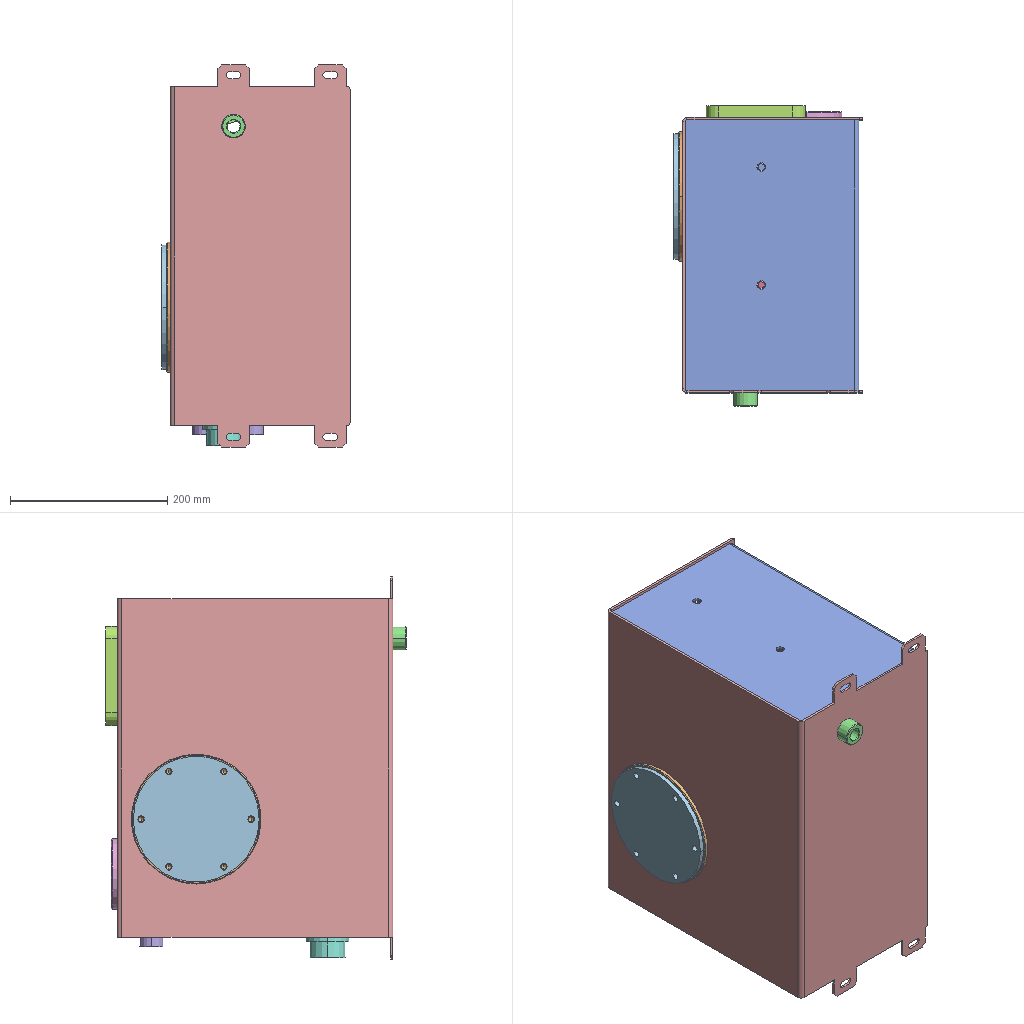Assembly | SolidWorks | 11 different items | 13 placed | box 239 x 382 x 486 mm
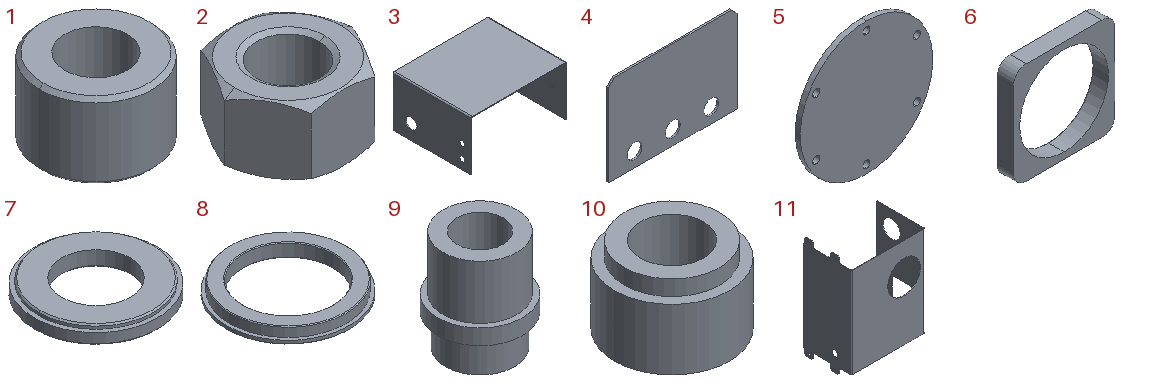Parts list (item | quantity | size | volume | features):
1 | x1 | 30 x 30 x 20 mm | 9753 mm3 | features Chamfer 2, HoleWzd 1, Revolution 1
2 | x2 | 27.713 x 24 x 14.8 mm | 5071 mm3 | features RevCut 2, Chamfer 1, Extrusion 1, LPattern 1
3 | x1 | 422 x 344 x 221 mm | 872945 mm3 | features ICE 2, Fillet 1, FlatPattern 1, SMBaseFlange 1, SheetMetal 1, UnFold 1
4 | x1 | 218 x 3 x 150 mm | 93382 mm3 | features FlatPattern 1, SMBaseFlange 1, SheetMetal 1
5 | x1 | 160 x 6 x 160 mm | 118594 mm3 | features FlatPattern 1, SMBaseFlange 1, SheetMetal 1
6 | x1 | 126 x 20 x 126 mm | 119235 mm3 | features Chamfer 1, Extrusion 1, HoleWzd 1, ICE 1
7 | x1 | 90 x 90 x 11 mm | 45138 mm3 | features Chamfer 2, HoleWzd 1, ICE 1, Revolution 1
8 | x1 | 165 x 165 x 18 mm | 148586 mm3 | features Chamfer 2, HoleWzd 1, ICE 1, Revolution 1
9 | x1 | 55 x 55 x 65 mm | 76144 mm3 | features HoleWzd 1, Revolution 1
10 | x2 | 30 x 30 x 20 mm | 8982 mm3 | features Chamfer 1, HoleWzd 1, Revolution 1
11 | x1 | 350 x 228 x 486 mm | 915789 mm3 | features ICE 5, Chamfer 1, Fillet 1, FlatPattern 1, SMBaseFlange 1, SheetMetal 1, UnFold 1
Mates (type | each side: item.copy, entity, surface, feature):
Coincident | 11.1 face plane Base-Flange1 | 3.1 face plane Base-Flange1 | 2 times
DistanceDim | 3.1 face plane Base-Flange1 | 11.1 face plane Cut-Extrude3
Coincident | 11.1 face plane Cut-Extrude4 | 6.1 face plane Boss-Extrude1 | 2 times
DistanceDim | 6.1 face plane Boss-Extrude1 | 11.1 face plane Base-Flange1
Concentric | 11.1 face cylinder Cut-Extrude4 | 7.1 face cylinder Revolve1
Coincident | 11.1 face plane Base-Flange1 | 7.1 face plane Revolve1
Perpendicular | 11.1 plane | 7.1 plane
Concentric | 3.1 face cylinder Cut-Extrude2 | 9.1 face cylinder Revolve1
Coincident | 3.1 face plane Base-Flange1 | 9.1 face plane Revolve1
Concentric | 11.1 face cylinder Cut-Extrude1 | 8.1 face cylinder Revolve1
Coincident | 11.1 face plane Base-Flange1 | 8.1 face plane Revolve1
Parallel | 11.1 plane | 8.1 plane
Concentric | 3.1 face cylinder Cut-Extrude2 | 10.1 face cylinder Revolve1
Coincident | 3.1 face plane Base-Flange1 | 10.1 face plane Revolve1
Concentric | 3.1 face cylinder Cut-Extrude2 | 10.2 face cylinder Revolve1
Coincident | 3.1 face plane Base-Flange1 | 10.2 face plane Revolve1
Concentric | 11.1 face cylinder Cut-Extrude5 | 1.1 face cylinder Revolve1
DistanceDim | 1.1 face plane Revolve1 | 11.1 face plane Base-Flange1
Coincident | 3.1 face plane Base-Flange1 | 4.1 face plane Base-Flange1 | 2 times
DistanceDim | 4.1 face plane Base-Flange1 | 3.1 face plane Base-Flange1
Concentric | 3.1 face cylinder Cut-Extrude1 | 2.1 face cone EndChamfer
Coincident | 3.1 face plane Base-Flange1 | 2.1 face plane BaseNut
Concentric | 3.1 face cylinder Cut-Extrude1 | 2.2 face cone EndChamfer
Coincident | 3.1 face plane Base-Flange1 | 2.2 face plane BaseNut
Coincident | 8.1 face plane Revolve1 | 5.1 face plane Base-Flange1
Concentric | 8.1 face cylinder M8 Tapped Hole1 | 5.1 face cylinder Base-Flange1 | 2 times